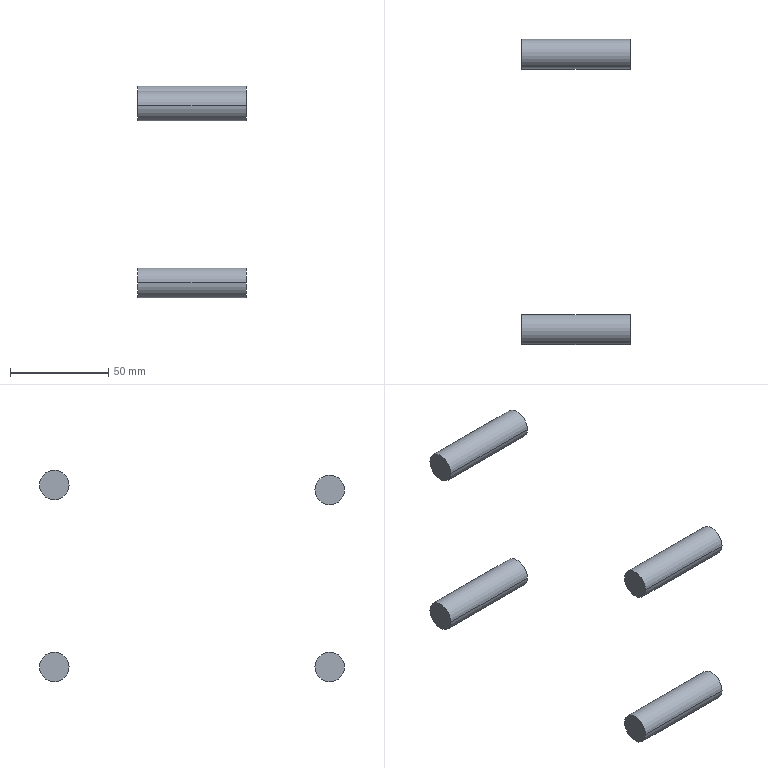Part | STEP file | PN_0012 | 4 solids | 16 faces | box 55 x 155 x 107.5 mm | volume 38877 mm3 | plane 8 | cylinder 8 | commonest cylinder face diameters 15 x8
STEP:
#1=CARTESIAN_POINT('',(0.,0.,0.));
#2=DIRECTION('',(0.,0.,1.));
#3=DIRECTION('',(1.,0.,0.));
#4=AXIS2_PLACEMENT_3D('',#1,#2,#3);
#5=CARTESIAN_POINT('',(124.2,-77.5,47.));
#6=VERTEX_POINT('',#5);
#7=CARTESIAN_POINT('',(124.2,-62.5,47.));
#8=VERTEX_POINT('',#7);
#9=CARTESIAN_POINT('',(124.2,-70.,47.));
#10=DIRECTION('',(-1.,0.,0.));
#11=DIRECTION('',(0.,-1.,0.));
#12=AXIS2_PLACEMENT_3D('',#9,#10,#11);
#13=CIRCLE('',#12,7.5);
#14=CARTESIAN_POINT('',(124.2,0.,0.));
#15=DIRECTION('',(-1.,0.,0.));
#16=DIRECTION('',(0.,-1.,0.));
#17=AXIS2_PLACEMENT_3D('',#14,#15,#16);
#18=PLANE('',#17);
#19=CARTESIAN_POINT('',(70.,47.));
#20=DIRECTION('',(1.,0.));
#21=AXIS2_PLACEMENT_2D('',#19,#20);
#22=CIRCLE('',#21,7.5);
#23=(GEOMETRIC_REPRESENTATION_CONTEXT(2)PARAMETRIC_REPRESENTATION_CONTEXT()REPRESENTATION_CONTEXT('',''));
#24=DEFINITIONAL_REPRESENTATION('',(#22),#23);
#25=PCURVE('',#18,#24);
#26=CARTESIAN_POINT('',(124.2,-70.,47.));
#27=DIRECTION('',(-1.,0.,0.));
#28=DIRECTION('',(0.,-1.,0.));
#29=AXIS2_PLACEMENT_3D('',#26,#27,#28);
#30=CYLINDRICAL_SURFACE('',#29,7.5);
#31=CARTESIAN_POINT('',(0.,0.));
#32=DIRECTION('',(1.,0.));
#33=VECTOR('',#32,1.);
#34=LINE('',#31,#33);
#35=(GEOMETRIC_REPRESENTATION_CONTEXT(2)PARAMETRIC_REPRESENTATION_CONTEXT()REPRESENTATION_CONTEXT('',''));
#36=DEFINITIONAL_REPRESENTATION('',(#34),#35);
#37=PCURVE('',#30,#36);
#38=SURFACE_CURVE('',#13,(#25,#37),.PCURVE_S1.);
#39=EDGE_CURVE('',#6,#8,#38,.T.);
#40=ORIENTED_EDGE('',*,*,#39,.T.);
#41=CARTESIAN_POINT('',(124.2,-70.,47.));
#42=DIRECTION('',(-1.,0.,0.));
#43=DIRECTION('',(0.,1.,0.));
#44=AXIS2_PLACEMENT_3D('',#41,#42,#43);
#45=CIRCLE('',#44,7.5);
#46=CARTESIAN_POINT('',(70.,47.));
#47=DIRECTION('',(-1.,0.));
#48=AXIS2_PLACEMENT_2D('',#46,#47);
#49=CIRCLE('',#48,7.5);
#50=(GEOMETRIC_REPRESENTATION_CONTEXT(2)PARAMETRIC_REPRESENTATION_CONTEXT()REPRESENTATION_CONTEXT('',''));
#51=DEFINITIONAL_REPRESENTATION('',(#49),#50);
#52=PCURVE('',#18,#51);
#53=CARTESIAN_POINT('',(124.2,-70.,47.));
#54=DIRECTION('',(-1.,0.,0.));
#55=DIRECTION('',(0.,-1.,0.));
#56=AXIS2_PLACEMENT_3D('',#53,#54,#55);
#57=CYLINDRICAL_SURFACE('',#56,7.5);
#58=CARTESIAN_POINT('',(3.142,0.));
#59=DIRECTION('',(1.,0.));
#60=VECTOR('',#59,1.);
#61=LINE('',#58,#60);
#62=(GEOMETRIC_REPRESENTATION_CONTEXT(2)PARAMETRIC_REPRESENTATION_CONTEXT()REPRESENTATION_CONTEXT('',''));
#63=DEFINITIONAL_REPRESENTATION('',(#61),#62);
#64=PCURVE('',#57,#63);
#65=SURFACE_CURVE('',#45,(#52,#64),.PCURVE_S1.);
#66=EDGE_CURVE('',#8,#6,#65,.T.);
#67=ORIENTED_EDGE('',*,*,#66,.T.);
#68=EDGE_LOOP('',(#40,#67));
#69=FACE_BOUND('',#68,.F.);
#70=ADVANCED_FACE('',(#69),#18,.F.);
#71=CARTESIAN_POINT('',(69.2,-62.5,47.));
#72=VERTEX_POINT('',#71);
#73=CARTESIAN_POINT('',(124.2,-62.5,47.));
#74=DIRECTION('',(-1.,0.,0.));
#75=VECTOR('',#74,1.);
#76=LINE('',#73,#75);
#77=CARTESIAN_POINT('',(3.142,0.));
#78=DIRECTION('',(0.,1.));
#79=VECTOR('',#78,1.);
#80=LINE('',#77,#79);
#81=(GEOMETRIC_REPRESENTATION_CONTEXT(2)PARAMETRIC_REPRESENTATION_CONTEXT()REPRESENTATION_CONTEXT('',''));
#82=DEFINITIONAL_REPRESENTATION('',(#80),#81);
#83=PCURVE('',#30,#82);
#84=CARTESIAN_POINT('',(3.142,0.));
#85=DIRECTION('',(0.,1.));
#86=VECTOR('',#85,1.);
#87=LINE('',#84,#86);
#88=(GEOMETRIC_REPRESENTATION_CONTEXT(2)PARAMETRIC_REPRESENTATION_CONTEXT()REPRESENTATION_CONTEXT('',''));
#89=DEFINITIONAL_REPRESENTATION('',(#87),#88);
#90=PCURVE('',#57,#89);
#91=SURFACE_CURVE('',#76,(#83,#90),.PCURVE_S1.);
#92=EDGE_CURVE('',#8,#72,#91,.T.);
#93=ORIENTED_EDGE('',*,*,#92,.T.);
#94=CARTESIAN_POINT('',(69.2,-77.5,47.));
#95=VERTEX_POINT('',#94);
#96=CARTESIAN_POINT('',(69.2,-70.,47.));
#97=DIRECTION('',(-1.,0.,0.));
#98=DIRECTION('',(0.,-1.,0.));
#99=AXIS2_PLACEMENT_3D('',#96,#97,#98);
#100=CIRCLE('',#99,7.5);
#101=CARTESIAN_POINT('',(0.,55.));
#102=DIRECTION('',(1.,0.));
#103=VECTOR('',#102,1.);
#104=LINE('',#101,#103);
#105=(GEOMETRIC_REPRESENTATION_CONTEXT(2)PARAMETRIC_REPRESENTATION_CONTEXT()REPRESENTATION_CONTEXT('',''));
#106=DEFINITIONAL_REPRESENTATION('',(#104),#105);
#107=PCURVE('',#30,#106);
#108=CARTESIAN_POINT('',(69.2,0.,0.));
#109=DIRECTION('',(-1.,0.,0.));
#110=DIRECTION('',(0.,-1.,0.));
#111=AXIS2_PLACEMENT_3D('',#108,#109,#110);
#112=PLANE('',#111);
#113=CARTESIAN_POINT('',(70.,47.));
#114=DIRECTION('',(1.,0.));
#115=AXIS2_PLACEMENT_2D('',#113,#114);
#116=CIRCLE('',#115,7.5);
#117=(GEOMETRIC_REPRESENTATION_CONTEXT(2)PARAMETRIC_REPRESENTATION_CONTEXT()REPRESENTATION_CONTEXT('',''));
#118=DEFINITIONAL_REPRESENTATION('',(#116),#117);
#119=PCURVE('',#112,#118);
#120=SURFACE_CURVE('',#100,(#107,#119),.PCURVE_S1.);
#121=EDGE_CURVE('',#95,#72,#120,.T.);
#122=ORIENTED_EDGE('',*,*,#121,.F.);
#123=CARTESIAN_POINT('',(124.2,-77.5,47.));
#124=DIRECTION('',(-1.,0.,0.));
#125=VECTOR('',#124,1.);
#126=LINE('',#123,#125);
#127=CARTESIAN_POINT('',(0.,0.));
#128=DIRECTION('',(0.,1.));
#129=VECTOR('',#128,1.);
#130=LINE('',#127,#129);
#131=(GEOMETRIC_REPRESENTATION_CONTEXT(2)PARAMETRIC_REPRESENTATION_CONTEXT()REPRESENTATION_CONTEXT('',''));
#132=DEFINITIONAL_REPRESENTATION('',(#130),#131);
#133=PCURVE('',#30,#132);
#134=CARTESIAN_POINT('',(6.283,0.));
#135=DIRECTION('',(0.,1.));
#136=VECTOR('',#135,1.);
#137=LINE('',#134,#136);
#138=(GEOMETRIC_REPRESENTATION_CONTEXT(2)PARAMETRIC_REPRESENTATION_CONTEXT()REPRESENTATION_CONTEXT('',''));
#139=DEFINITIONAL_REPRESENTATION('',(#137),#138);
#140=PCURVE('',#57,#139);
#141=SURFACE_CURVE('',#126,(#133,#140),.PCURVE_S1.);
#142=EDGE_CURVE('',#6,#95,#141,.T.);
#143=ORIENTED_EDGE('',*,*,#142,.F.);
#144=ORIENTED_EDGE('',*,*,#39,.T.);
#145=EDGE_LOOP('',(#93,#122,#143,#144));
#146=FACE_BOUND('',#145,.T.);
#147=ADVANCED_FACE('',(#146),#30,.T.);
#148=ORIENTED_EDGE('',*,*,#142,.T.);
#149=CARTESIAN_POINT('',(69.2,-70.,47.));
#150=DIRECTION('',(-1.,0.,0.));
#151=DIRECTION('',(0.,1.,0.));
#152=AXIS2_PLACEMENT_3D('',#149,#150,#151);
#153=CIRCLE('',#152,7.5);
#154=CARTESIAN_POINT('',(3.142,55.));
#155=DIRECTION('',(1.,0.));
#156=VECTOR('',#155,1.);
#157=LINE('',#154,#156);
#158=(GEOMETRIC_REPRESENTATION_CONTEXT(2)PARAMETRIC_REPRESENTATION_CONTEXT()REPRESENTATION_CONTEXT('',''));
#159=DEFINITIONAL_REPRESENTATION('',(#157),#158);
#160=PCURVE('',#57,#159);
#161=CARTESIAN_POINT('',(70.,47.));
#162=DIRECTION('',(-1.,0.));
#163=AXIS2_PLACEMENT_2D('',#161,#162);
#164=CIRCLE('',#163,7.5);
#165=(GEOMETRIC_REPRESENTATION_CONTEXT(2)PARAMETRIC_REPRESENTATION_CONTEXT()REPRESENTATION_CONTEXT('',''));
#166=DEFINITIONAL_REPRESENTATION('',(#164),#165);
#167=PCURVE('',#112,#166);
#168=SURFACE_CURVE('',#153,(#160,#167),.PCURVE_S1.);
#169=EDGE_CURVE('',#72,#95,#168,.T.);
#170=ORIENTED_EDGE('',*,*,#169,.F.);
#171=ORIENTED_EDGE('',*,*,#92,.F.);
#172=ORIENTED_EDGE('',*,*,#66,.T.);
#173=EDGE_LOOP('',(#148,#170,#171,#172));
#174=FACE_BOUND('',#173,.T.);
#175=ADVANCED_FACE('',(#174),#57,.T.);
#176=ORIENTED_EDGE('',*,*,#121,.F.);
#177=ORIENTED_EDGE('',*,*,#169,.F.);
#178=EDGE_LOOP('',(#176,#177));
#179=FACE_BOUND('',#178,.F.);
#180=ADVANCED_FACE('',(#179),#112,.T.);
#181=CLOSED_SHELL('',(#70,#147,#175,#180));
#182=MANIFOLD_SOLID_BREP('',#181);
#183=CARTESIAN_POINT('',(124.2,62.5,49.5));
#184=VERTEX_POINT('',#183);
#185=CARTESIAN_POINT('',(124.2,77.5,49.5));
#186=VERTEX_POINT('',#185);
#187=CARTESIAN_POINT('',(124.2,70.,49.5));
#188=DIRECTION('',(-1.,0.,0.));
#189=DIRECTION('',(0.,-1.,0.));
#190=AXIS2_PLACEMENT_3D('',#187,#188,#189);
#191=CIRCLE('',#190,7.5);
#192=CARTESIAN_POINT('',(124.2,0.,0.));
#193=DIRECTION('',(-1.,0.,0.));
#194=DIRECTION('',(0.,-1.,0.));
#195=AXIS2_PLACEMENT_3D('',#192,#193,#194);
#196=PLANE('',#195);
#197=CARTESIAN_POINT('',(-70.,49.5));
#198=DIRECTION('',(1.,0.));
#199=AXIS2_PLACEMENT_2D('',#197,#198);
#200=CIRCLE('',#199,7.5);
#201=(GEOMETRIC_REPRESENTATION_CONTEXT(2)PARAMETRIC_REPRESENTATION_CONTEXT()REPRESENTATION_CONTEXT('',''));
#202=DEFINITIONAL_REPRESENTATION('',(#200),#201);
#203=PCURVE('',#196,#202);
#204=CARTESIAN_POINT('',(124.2,70.,49.5));
#205=DIRECTION('',(-1.,0.,0.));
#206=DIRECTION('',(0.,-1.,0.));
#207=AXIS2_PLACEMENT_3D('',#204,#205,#206);
#208=CYLINDRICAL_SURFACE('',#207,7.5);
#209=CARTESIAN_POINT('',(0.,0.));
#210=DIRECTION('',(1.,0.));
#211=VECTOR('',#210,1.);
#212=LINE('',#209,#211);
#213=(GEOMETRIC_REPRESENTATION_CONTEXT(2)PARAMETRIC_REPRESENTATION_CONTEXT()REPRESENTATION_CONTEXT('',''));
#214=DEFINITIONAL_REPRESENTATION('',(#212),#213);
#215=PCURVE('',#208,#214);
#216=SURFACE_CURVE('',#191,(#203,#215),.PCURVE_S1.);
#217=EDGE_CURVE('',#184,#186,#216,.T.);
#218=ORIENTED_EDGE('',*,*,#217,.T.);
#219=CARTESIAN_POINT('',(124.2,70.,49.5));
#220=DIRECTION('',(-1.,0.,0.));
#221=DIRECTION('',(0.,1.,0.));
#222=AXIS2_PLACEMENT_3D('',#219,#220,#221);
#223=CIRCLE('',#222,7.5);
#224=CARTESIAN_POINT('',(-70.,49.5));
#225=DIRECTION('',(-1.,0.));
#226=AXIS2_PLACEMENT_2D('',#224,#225);
#227=CIRCLE('',#226,7.5);
#228=(GEOMETRIC_REPRESENTATION_CONTEXT(2)PARAMETRIC_REPRESENTATION_CONTEXT()REPRESENTATION_CONTEXT('',''));
#229=DEFINITIONAL_REPRESENTATION('',(#227),#228);
#230=PCURVE('',#196,#229);
#231=CARTESIAN_POINT('',(124.2,70.,49.5));
#232=DIRECTION('',(-1.,0.,0.));
#233=DIRECTION('',(0.,-1.,0.));
#234=AXIS2_PLACEMENT_3D('',#231,#232,#233);
#235=CYLINDRICAL_SURFACE('',#234,7.5);
#236=CARTESIAN_POINT('',(3.142,0.));
#237=DIRECTION('',(1.,0.));
#238=VECTOR('',#237,1.);
#239=LINE('',#236,#238);
#240=(GEOMETRIC_REPRESENTATION_CONTEXT(2)PARAMETRIC_REPRESENTATION_CONTEXT()REPRESENTATION_CONTEXT('',''));
#241=DEFINITIONAL_REPRESENTATION('',(#239),#240);
#242=PCURVE('',#235,#241);
#243=SURFACE_CURVE('',#223,(#230,#242),.PCURVE_S1.);
#244=EDGE_CURVE('',#186,#184,#243,.T.);
#245=ORIENTED_EDGE('',*,*,#244,.T.);
#246=EDGE_LOOP('',(#218,#245));
#247=FACE_BOUND('',#246,.F.);
#248=ADVANCED_FACE('',(#247),#196,.F.);
#249=CARTESIAN_POINT('',(69.2,77.5,49.5));
#250=VERTEX_POINT('',#249);
#251=CARTESIAN_POINT('',(124.2,77.5,49.5));
#252=DIRECTION('',(-1.,0.,0.));
#253=VECTOR('',#252,1.);
#254=LINE('',#251,#253);
#255=CARTESIAN_POINT('',(3.142,0.));
#256=DIRECTION('',(0.,1.));
#257=VECTOR('',#256,1.);
#258=LINE('',#255,#257);
#259=(GEOMETRIC_REPRESENTATION_CONTEXT(2)PARAMETRIC_REPRESENTATION_CONTEXT()REPRESENTATION_CONTEXT('',''));
#260=DEFINITIONAL_REPRESENTATION('',(#258),#259);
#261=PCURVE('',#208,#260);
#262=CARTESIAN_POINT('',(3.142,0.));
#263=DIRECTION('',(0.,1.));
#264=VECTOR('',#263,1.);
#265=LINE('',#262,#264);
#266=(GEOMETRIC_REPRESENTATION_CONTEXT(2)PARAMETRIC_REPRESENTATION_CONTEXT()REPRESENTATION_CONTEXT('',''));
#267=DEFINITIONAL_REPRESENTATION('',(#265),#266);
#268=PCURVE('',#235,#267);
#269=SURFACE_CURVE('',#254,(#261,#268),.PCURVE_S1.);
#270=EDGE_CURVE('',#186,#250,#269,.T.);
#271=ORIENTED_EDGE('',*,*,#270,.T.);
#272=CARTESIAN_POINT('',(69.2,62.5,49.5));
#273=VERTEX_POINT('',#272);
#274=CARTESIAN_POINT('',(69.2,70.,49.5));
#275=DIRECTION('',(-1.,0.,0.));
#276=DIRECTION('',(0.,-1.,0.));
#277=AXIS2_PLACEMENT_3D('',#274,#275,#276);
#278=CIRCLE('',#277,7.5);
#279=CARTESIAN_POINT('',(0.,55.));
#280=DIRECTION('',(1.,0.));
#281=VECTOR('',#280,1.);
#282=LINE('',#279,#281);
#283=(GEOMETRIC_REPRESENTATION_CONTEXT(2)PARAMETRIC_REPRESENTATION_CONTEXT()REPRESENTATION_CONTEXT('',''));
#284=DEFINITIONAL_REPRESENTATION('',(#282),#283);
#285=PCURVE('',#208,#284);
#286=CARTESIAN_POINT('',(69.2,0.,0.));
#287=DIRECTION('',(-1.,0.,0.));
#288=DIRECTION('',(0.,-1.,0.));
#289=AXIS2_PLACEMENT_3D('',#286,#287,#288);
#290=PLANE('',#289);
#291=CARTESIAN_POINT('',(-70.,49.5));
#292=DIRECTION('',(1.,0.));
#293=AXIS2_PLACEMENT_2D('',#291,#292);
#294=CIRCLE('',#293,7.5);
#295=(GEOMETRIC_REPRESENTATION_CONTEXT(2)PARAMETRIC_REPRESENTATION_CONTEXT()REPRESENTATION_CONTEXT('',''));
#296=DEFINITIONAL_REPRESENTATION('',(#294),#295);
#297=PCURVE('',#290,#296);
#298=SURFACE_CURVE('',#278,(#285,#297),.PCURVE_S1.);
#299=EDGE_CURVE('',#273,#250,#298,.T.);
#300=ORIENTED_EDGE('',*,*,#299,.F.);
#301=CARTESIAN_POINT('',(124.2,62.5,49.5));
#302=DIRECTION('',(-1.,0.,0.));
#303=VECTOR('',#302,1.);
#304=LINE('',#301,#303);
#305=CARTESIAN_POINT('',(0.,0.));
#306=DIRECTION('',(0.,1.));
#307=VECTOR('',#306,1.);
#308=LINE('',#305,#307);
#309=(GEOMETRIC_REPRESENTATION_CONTEXT(2)PARAMETRIC_REPRESENTATION_CONTEXT()REPRESENTATION_CONTEXT('',''));
#310=DEFINITIONAL_REPRESENTATION('',(#308),#309);
#311=PCURVE('',#208,#310);
#312=CARTESIAN_POINT('',(6.283,0.));
#313=DIRECTION('',(0.,1.));
#314=VECTOR('',#313,1.);
#315=LINE('',#312,#314);
#316=(GEOMETRIC_REPRESENTATION_CONTEXT(2)PARAMETRIC_REPRESENTATION_CONTEXT()REPRESENTATION_CONTEXT('',''));
#317=DEFINITIONAL_REPRESENTATION('',(#315),#316);
#318=PCURVE('',#235,#317);
#319=SURFACE_CURVE('',#304,(#311,#318),.PCURVE_S1.);
#320=EDGE_CURVE('',#184,#273,#319,.T.);
#321=ORIENTED_EDGE('',*,*,#320,.F.);
#322=ORIENTED_EDGE('',*,*,#217,.T.);
#323=EDGE_LOOP('',(#271,#300,#321,#322));
#324=FACE_BOUND('',#323,.T.);
#325=ADVANCED_FACE('',(#324),#208,.T.);
#326=ORIENTED_EDGE('',*,*,#320,.T.);
#327=CARTESIAN_POINT('',(69.2,70.,49.5));
#328=DIRECTION('',(-1.,0.,0.));
#329=DIRECTION('',(0.,1.,0.));
#330=AXIS2_PLACEMENT_3D('',#327,#328,#329);
#331=CIRCLE('',#330,7.5);
#332=CARTESIAN_POINT('',(3.142,55.));
#333=DIRECTION('',(1.,0.));
#334=VECTOR('',#333,1.);
#335=LINE('',#332,#334);
#336=(GEOMETRIC_REPRESENTATION_CONTEXT(2)PARAMETRIC_REPRESENTATION_CONTEXT()REPRESENTATION_CONTEXT('',''));
#337=DEFINITIONAL_REPRESENTATION('',(#335),#336);
#338=PCURVE('',#235,#337);
#339=CARTESIAN_POINT('',(-70.,49.5));
#340=DIRECTION('',(-1.,0.));
#341=AXIS2_PLACEMENT_2D('',#339,#340);
#342=CIRCLE('',#341,7.5);
#343=(GEOMETRIC_REPRESENTATION_CONTEXT(2)PARAMETRIC_REPRESENTATION_CONTEXT()REPRESENTATION_CONTEXT('',''));
#344=DEFINITIONAL_REPRESENTATION('',(#342),#343);
#345=PCURVE('',#290,#344);
#346=SURFACE_CURVE('',#331,(#338,#345),.PCURVE_S1.);
#347=EDGE_CURVE('',#250,#273,#346,.T.);
#348=ORIENTED_EDGE('',*,*,#347,.F.);
#349=ORIENTED_EDGE('',*,*,#270,.F.);
#350=ORIENTED_EDGE('',*,*,#244,.T.);
#351=EDGE_LOOP('',(#326,#348,#349,#350));
#352=FACE_BOUND('',#351,.T.);
#353=ADVANCED_FACE('',(#352),#235,.T.);
#354=ORIENTED_EDGE('',*,*,#299,.F.);
#355=ORIENTED_EDGE('',*,*,#347,.F.);
#356=EDGE_LOOP('',(#354,#355));
#357=FACE_BOUND('',#356,.F.);
#358=ADVANCED_FACE('',(#357),#290,.T.);
#359=CLOSED_SHELL('',(#248,#325,#353,#358));
#360=MANIFOLD_SOLID_BREP('',#359);
#361=CARTESIAN_POINT('',(124.2,62.5,-43.));
#362=VERTEX_POINT('',#361);
#363=CARTESIAN_POINT('',(124.2,77.5,-43.));
#364=VERTEX_POINT('',#363);
#365=CARTESIAN_POINT('',(124.2,70.,-43.));
#366=DIRECTION('',(-1.,0.,0.));
#367=DIRECTION('',(0.,-1.,0.));
#368=AXIS2_PLACEMENT_3D('',#365,#366,#367);
#369=CIRCLE('',#368,7.5);
#370=CARTESIAN_POINT('',(124.2,0.,0.));
#371=DIRECTION('',(-1.,0.,0.));
#372=DIRECTION('',(0.,-1.,0.));
#373=AXIS2_PLACEMENT_3D('',#370,#371,#372);
#374=PLANE('',#373);
#375=CARTESIAN_POINT('',(-70.,-43.));
#376=DIRECTION('',(1.,0.));
#377=AXIS2_PLACEMENT_2D('',#375,#376);
#378=CIRCLE('',#377,7.5);
#379=(GEOMETRIC_REPRESENTATION_CONTEXT(2)PARAMETRIC_REPRESENTATION_CONTEXT()REPRESENTATION_CONTEXT('',''));
#380=DEFINITIONAL_REPRESENTATION('',(#378),#379);
#381=PCURVE('',#374,#380);
#382=CARTESIAN_POINT('',(124.2,70.,-43.));
#383=DIRECTION('',(-1.,0.,0.));
#384=DIRECTION('',(0.,-1.,0.));
#385=AXIS2_PLACEMENT_3D('',#382,#383,#384);
#386=CYLINDRICAL_SURFACE('',#385,7.5);
#387=CARTESIAN_POINT('',(0.,0.));
#388=DIRECTION('',(1.,0.));
#389=VECTOR('',#388,1.);
#390=LINE('',#387,#389);
#391=(GEOMETRIC_REPRESENTATION_CONTEXT(2)PARAMETRIC_REPRESENTATION_CONTEXT()REPRESENTATION_CONTEXT('',''));
#392=DEFINITIONAL_REPRESENTATION('',(#390),#391);
#393=PCURVE('',#386,#392);
#394=SURFACE_CURVE('',#369,(#381,#393),.PCURVE_S1.);
#395=EDGE_CURVE('',#362,#364,#394,.T.);
#396=ORIENTED_EDGE('',*,*,#395,.T.);
#397=CARTESIAN_POINT('',(124.2,70.,-43.));
#398=DIRECTION('',(-1.,0.,0.));
#399=DIRECTION('',(0.,1.,0.));
#400=AXIS2_PLACEMENT_3D('',#397,#398,#399);
#401=CIRCLE('',#400,7.5);
#402=CARTESIAN_POINT('',(-70.,-43.));
#403=DIRECTION('',(-1.,0.));
#404=AXIS2_PLACEMENT_2D('',#402,#403);
#405=CIRCLE('',#404,7.5);
#406=(GEOMETRIC_REPRESENTATION_CONTEXT(2)PARAMETRIC_REPRESENTATION_CONTEXT()REPRESENTATION_CONTEXT('',''));
#407=DEFINITIONAL_REPRESENTATION('',(#405),#406);
#408=PCURVE('',#374,#407);
#409=CARTESIAN_POINT('',(124.2,70.,-43.));
#410=DIRECTION('',(-1.,0.,0.));
#411=DIRECTION('',(0.,-1.,0.));
#412=AXIS2_PLACEMENT_3D('',#409,#410,#411);
#413=CYLINDRICAL_SURFACE('',#412,7.5);
#414=CARTESIAN_POINT('',(3.142,0.));
#415=DIRECTION('',(1.,0.));
#416=VECTOR('',#415,1.);
#417=LINE('',#414,#416);
#418=(GEOMETRIC_REPRESENTATION_CONTEXT(2)PARAMETRIC_REPRESENTATION_CONTEXT()REPRESENTATION_CONTEXT('',''));
#419=DEFINITIONAL_REPRESENTATION('',(#417),#418);
#420=PCURVE('',#413,#419);
#421=SURFACE_CURVE('',#401,(#408,#420),.PCURVE_S1.);
#422=EDGE_CURVE('',#364,#362,#421,.T.);
#423=ORIENTED_EDGE('',*,*,#422,.T.);
#424=EDGE_LOOP('',(#396,#423));
#425=FACE_BOUND('',#424,.F.);
#426=ADVANCED_FACE('',(#425),#374,.F.);
#427=CARTESIAN_POINT('',(69.2,77.5,-43.));
#428=VERTEX_POINT('',#427);
#429=CARTESIAN_POINT('',(124.2,77.5,-43.));
#430=DIRECTION('',(-1.,0.,0.));
#431=VECTOR('',#430,1.);
#432=LINE('',#429,#431);
#433=CARTESIAN_POINT('',(3.142,0.));
#434=DIRECTION('',(0.,1.));
#435=VECTOR('',#434,1.);
#436=LINE('',#433,#435);
#437=(GEOMETRIC_REPRESENTATION_CONTEXT(2)PARAMETRIC_REPRESENTATION_CONTEXT()REPRESENTATION_CONTEXT('',''));
#438=DEFINITIONAL_REPRESENTATION('',(#436),#437);
#439=PCURVE('',#386,#438);
#440=CARTESIAN_POINT('',(3.142,0.));
#441=DIRECTION('',(0.,1.));
#442=VECTOR('',#441,1.);
#443=LINE('',#440,#442);
#444=(GEOMETRIC_REPRESENTATION_CONTEXT(2)PARAMETRIC_REPRESENTATION_CONTEXT()REPRESENTATION_CONTEXT('',''));
#445=DEFINITIONAL_REPRESENTATION('',(#443),#444);
#446=PCURVE('',#413,#445);
#447=SURFACE_CURVE('',#432,(#439,#446),.PCURVE_S1.);
#448=EDGE_CURVE('',#364,#428,#447,.T.);
#449=ORIENTED_EDGE('',*,*,#448,.T.);
#450=CARTESIAN_POINT('',(69.2,62.5,-43.));
#451=VERTEX_POINT('',#450);
#452=CARTESIAN_POINT('',(69.2,70.,-43.));
#453=DIRECTION('',(-1.,0.,0.));
#454=DIRECTION('',(0.,-1.,0.));
#455=AXIS2_PLACEMENT_3D('',#452,#453,#454);
#456=CIRCLE('',#455,7.5);
#457=CARTESIAN_POINT('',(0.,55.));
#458=DIRECTION('',(1.,0.));
#459=VECTOR('',#458,1.);
#460=LINE('',#457,#459);
#461=(GEOMETRIC_REPRESENTATION_CONTEXT(2)PARAMETRIC_REPRESENTATION_CONTEXT()REPRESENTATION_CONTEXT('',''));
#462=DEFINITIONAL_REPRESENTATION('',(#460),#461);
#463=PCURVE('',#386,#462);
#464=CARTESIAN_POINT('',(69.2,0.,0.));
#465=DIRECTION('',(-1.,0.,0.));
#466=DIRECTION('',(0.,-1.,0.));
#467=AXIS2_PLACEMENT_3D('',#464,#465,#466);
#468=PLANE('',#467);
#469=CARTESIAN_POINT('',(-70.,-43.));
#470=DIRECTION('',(1.,0.));
#471=AXIS2_PLACEMENT_2D('',#469,#470);
#472=CIRCLE('',#471,7.5);
#473=(GEOMETRIC_REPRESENTATION_CONTEXT(2)PARAMETRIC_REPRESENTATION_CONTEXT()REPRESENTATION_CONTEXT('',''));
#474=DEFINITIONAL_REPRESENTATION('',(#472),#473);
#475=PCURVE('',#468,#474);
#476=SURFACE_CURVE('',#456,(#463,#475),.PCURVE_S1.);
#477=EDGE_CURVE('',#451,#428,#476,.T.);
#478=ORIENTED_EDGE('',*,*,#477,.F.);
#479=CARTESIAN_POINT('',(124.2,62.5,-43.));
#480=DIRECTION('',(-1.,0.,0.));
#481=VECTOR('',#480,1.);
#482=LINE('',#479,#481);
#483=CARTESIAN_POINT('',(0.,0.));
#484=DIRECTION('',(0.,1.));
#485=VECTOR('',#484,1.);
#486=LINE('',#483,#485);
#487=(GEOMETRIC_REPRESENTATION_CONTEXT(2)PARAMETRIC_REPRESENTATION_CONTEXT()REPRESENTATION_CONTEXT('',''));
#488=DEFINITIONAL_REPRESENTATION('',(#486),#487);
#489=PCURVE('',#386,#488);
#490=CARTESIAN_POINT('',(6.283,0.));
#491=DIRECTION('',(0.,1.));
#492=VECTOR('',#491,1.);
#493=LINE('',#490,#492);
#494=(GEOMETRIC_REPRESENTATION_CONTEXT(2)PARAMETRIC_REPRESENTATION_CONTEXT()REPRESENTATION_CONTEXT('',''));
#495=DEFINITIONAL_REPRESENTATION('',(#493),#494);
#496=PCURVE('',#413,#495);
#497=SURFACE_CURVE('',#482,(#489,#496),.PCURVE_S1.);
#498=EDGE_CURVE('',#362,#451,#497,.T.);
#499=ORIENTED_EDGE('',*,*,#498,.F.);
#500=ORIENTED_EDGE('',*,*,#395,.T.);
#501=EDGE_LOOP('',(#449,#478,#499,#500));
#502=FACE_BOUND('',#501,.T.);
#503=ADVANCED_FACE('',(#502),#386,.T.);
#504=ORIENTED_EDGE('',*,*,#498,.T.);
#505=CARTESIAN_POINT('',(69.2,70.,-43.));
#506=DIRECTION('',(-1.,0.,0.));
#507=DIRECTION('',(0.,1.,0.));
#508=AXIS2_PLACEMENT_3D('',#505,#506,#507);
#509=CIRCLE('',#508,7.5);
#510=CARTESIAN_POINT('',(3.142,55.));
#511=DIRECTION('',(1.,0.));
#512=VECTOR('',#511,1.);
#513=LINE('',#510,#512);
#514=(GEOMETRIC_REPRESENTATION_CONTEXT(2)PARAMETRIC_REPRESENTATION_CONTEXT()REPRESENTATION_CONTEXT('',''));
#515=DEFINITIONAL_REPRESENTATION('',(#513),#514);
#516=PCURVE('',#413,#515);
#517=CARTESIAN_POINT('',(-70.,-43.));
#518=DIRECTION('',(-1.,0.));
#519=AXIS2_PLACEMENT_2D('',#517,#518);
#520=CIRCLE('',#519,7.5);
#521=(GEOMETRIC_REPRESENTATION_CONTEXT(2)PARAMETRIC_REPRESENTATION_CONTEXT()REPRESENTATION_CONTEXT('',''));
#522=DEFINITIONAL_REPRESENTATION('',(#520),#521);
#523=PCURVE('',#468,#522);
#524=SURFACE_CURVE('',#509,(#516,#523),.PCURVE_S1.);
#525=EDGE_CURVE('',#428,#451,#524,.T.);
#526=ORIENTED_EDGE('',*,*,#525,.F.);
#527=ORIENTED_EDGE('',*,*,#448,.F.);
#528=ORIENTED_EDGE('',*,*,#422,.T.);
#529=EDGE_LOOP('',(#504,#526,#527,#528));
#530=FACE_BOUND('',#529,.T.);
#531=ADVANCED_FACE('',(#530),#413,.T.);
#532=ORIENTED_EDGE('',*,*,#477,.F.);
#533=ORIENTED_EDGE('',*,*,#525,.F.);
#534=EDGE_LOOP('',(#532,#533));
#535=FACE_BOUND('',#534,.F.);
#536=ADVANCED_FACE('',(#535),#468,.T.);
#537=CLOSED_SHELL('',(#426,#503,#531,#536));
#538=MANIFOLD_SOLID_BREP('',#537);
#539=CARTESIAN_POINT('',(124.2,-77.5,-43.));
#540=VERTEX_POINT('',#539);
#541=CARTESIAN_POINT('',(124.2,-62.5,-43.));
#542=VERTEX_POINT('',#541);
#543=CARTESIAN_POINT('',(124.2,-70.,-43.));
#544=DIRECTION('',(-1.,0.,0.));
#545=DIRECTION('',(0.,-1.,0.));
#546=AXIS2_PLACEMENT_3D('',#543,#544,#545);
#547=CIRCLE('',#546,7.5);
#548=CARTESIAN_POINT('',(124.2,0.,0.));
#549=DIRECTION('',(-1.,0.,0.));
#550=DIRECTION('',(0.,-1.,0.));
#551=AXIS2_PLACEMENT_3D('',#548,#549,#550);
#552=PLANE('',#551);
#553=CARTESIAN_POINT('',(70.,-43.));
#554=DIRECTION('',(1.,0.));
#555=AXIS2_PLACEMENT_2D('',#553,#554);
#556=CIRCLE('',#555,7.5);
#557=(GEOMETRIC_REPRESENTATION_CONTEXT(2)PARAMETRIC_REPRESENTATION_CONTEXT()REPRESENTATION_CONTEXT('',''));
#558=DEFINITIONAL_REPRESENTATION('',(#556),#557);
#559=PCURVE('',#552,#558);
#560=CARTESIAN_POINT('',(124.2,-70.,-43.));
#561=DIRECTION('',(-1.,0.,0.));
#562=DIRECTION('',(0.,-1.,0.));
#563=AXIS2_PLACEMENT_3D('',#560,#561,#562);
#564=CYLINDRICAL_SURFACE('',#563,7.5);
#565=CARTESIAN_POINT('',(0.,0.));
#566=DIRECTION('',(1.,0.));
#567=VECTOR('',#566,1.);
#568=LINE('',#565,#567);
#569=(GEOMETRIC_REPRESENTATION_CONTEXT(2)PARAMETRIC_REPRESENTATION_CONTEXT()REPRESENTATION_CONTEXT('',''));
#570=DEFINITIONAL_REPRESENTATION('',(#568),#569);
#571=PCURVE('',#564,#570);
#572=SURFACE_CURVE('',#547,(#559,#571),.PCURVE_S1.);
#573=EDGE_CURVE('',#540,#542,#572,.T.);
#574=ORIENTED_EDGE('',*,*,#573,.T.);
#575=CARTESIAN_POINT('',(124.2,-70.,-43.));
#576=DIRECTION('',(-1.,0.,0.));
#577=DIRECTION('',(0.,1.,0.));
#578=AXIS2_PLACEMENT_3D('',#575,#576,#577);
#579=CIRCLE('',#578,7.5);
#580=CARTESIAN_POINT('',(70.,-43.));
#581=DIRECTION('',(-1.,0.));
#582=AXIS2_PLACEMENT_2D('',#580,#581);
#583=CIRCLE('',#582,7.5);
#584=(GEOMETRIC_REPRESENTATION_CONTEXT(2)PARAMETRIC_REPRESENTATION_CONTEXT()REPRESENTATION_CONTEXT('',''));
#585=DEFINITIONAL_REPRESENTATION('',(#583),#584);
#586=PCURVE('',#552,#585);
#587=CARTESIAN_POINT('',(124.2,-70.,-43.));
#588=DIRECTION('',(-1.,0.,0.));
#589=DIRECTION('',(0.,-1.,0.));
#590=AXIS2_PLACEMENT_3D('',#587,#588,#589);
#591=CYLINDRICAL_SURFACE('',#590,7.5);
#592=CARTESIAN_POINT('',(3.142,0.));
#593=DIRECTION('',(1.,0.));
#594=VECTOR('',#593,1.);
#595=LINE('',#592,#594);
#596=(GEOMETRIC_REPRESENTATION_CONTEXT(2)PARAMETRIC_REPRESENTATION_CONTEXT()REPRESENTATION_CONTEXT('',''));
#597=DEFINITIONAL_REPRESENTATION('',(#595),#596);
#598=PCURVE('',#591,#597);
#599=SURFACE_CURVE('',#579,(#586,#598),.PCURVE_S1.);
#600=EDGE_CURVE('',#542,#540,#599,.T.);
#601=ORIENTED_EDGE('',*,*,#600,.T.);
#602=EDGE_LOOP('',(#574,#601));
#603=FACE_BOUND('',#602,.F.);
#604=ADVANCED_FACE('',(#603),#552,.F.);
#605=CARTESIAN_POINT('',(69.2,-62.5,-43.));
#606=VERTEX_POINT('',#605);
#607=CARTESIAN_POINT('',(124.2,-62.5,-43.));
#608=DIRECTION('',(-1.,0.,0.));
#609=VECTOR('',#608,1.);
#610=LINE('',#607,#609);
#611=CARTESIAN_POINT('',(3.142,0.));
#612=DIRECTION('',(0.,1.));
#613=VECTOR('',#612,1.);
#614=LINE('',#611,#613);
#615=(GEOMETRIC_REPRESENTATION_CONTEXT(2)PARAMETRIC_REPRESENTATION_CONTEXT()REPRESENTATION_CONTEXT('',''));
#616=DEFINITIONAL_REPRESENTATION('',(#614),#615);
#617=PCURVE('',#564,#616);
#618=CARTESIAN_POINT('',(3.142,0.));
#619=DIRECTION('',(0.,1.));
#620=VECTOR('',#619,1.);
#621=LINE('',#618,#620);
#622=(GEOMETRIC_REPRESENTATION_CONTEXT(2)PARAMETRIC_REPRESENTATION_CONTEXT()REPRESENTATION_CONTEXT('',''));
#623=DEFINITIONAL_REPRESENTATION('',(#621),#622);
#624=PCURVE('',#591,#623);
#625=SURFACE_CURVE('',#610,(#617,#624),.PCURVE_S1.);
#626=EDGE_CURVE('',#542,#606,#625,.T.);
#627=ORIENTED_EDGE('',*,*,#626,.T.);
#628=CARTESIAN_POINT('',(69.2,-77.5,-43.));
#629=VERTEX_POINT('',#628);
#630=CARTESIAN_POINT('',(69.2,-70.,-43.));
#631=DIRECTION('',(-1.,0.,0.));
#632=DIRECTION('',(0.,-1.,0.));
#633=AXIS2_PLACEMENT_3D('',#630,#631,#632);
#634=CIRCLE('',#633,7.5);
#635=CARTESIAN_POINT('',(0.,55.));
#636=DIRECTION('',(1.,0.));
#637=VECTOR('',#636,1.);
#638=LINE('',#635,#637);
#639=(GEOMETRIC_REPRESENTATION_CONTEXT(2)PARAMETRIC_REPRESENTATION_CONTEXT()REPRESENTATION_CONTEXT('',''));
#640=DEFINITIONAL_REPRESENTATION('',(#638),#639);
#641=PCURVE('',#564,#640);
#642=CARTESIAN_POINT('',(69.2,0.,0.));
#643=DIRECTION('',(-1.,0.,0.));
#644=DIRECTION('',(0.,-1.,0.));
#645=AXIS2_PLACEMENT_3D('',#642,#643,#644);
#646=PLANE('',#645);
#647=CARTESIAN_POINT('',(70.,-43.));
#648=DIRECTION('',(1.,0.));
#649=AXIS2_PLACEMENT_2D('',#647,#648);
#650=CIRCLE('',#649,7.5);
#651=(GEOMETRIC_REPRESENTATION_CONTEXT(2)PARAMETRIC_REPRESENTATION_CONTEXT()REPRESENTATION_CONTEXT('',''));
#652=DEFINITIONAL_REPRESENTATION('',(#650),#651);
#653=PCURVE('',#646,#652);
#654=SURFACE_CURVE('',#634,(#641,#653),.PCURVE_S1.);
#655=EDGE_CURVE('',#629,#606,#654,.T.);
#656=ORIENTED_EDGE('',*,*,#655,.F.);
#657=CARTESIAN_POINT('',(124.2,-77.5,-43.));
#658=DIRECTION('',(-1.,0.,0.));
#659=VECTOR('',#658,1.);
#660=LINE('',#657,#659);
#661=CARTESIAN_POINT('',(0.,0.));
#662=DIRECTION('',(0.,1.));
#663=VECTOR('',#662,1.);
#664=LINE('',#661,#663);
#665=(GEOMETRIC_REPRESENTATION_CONTEXT(2)PARAMETRIC_REPRESENTATION_CONTEXT()REPRESENTATION_CONTEXT('',''));
#666=DEFINITIONAL_REPRESENTATION('',(#664),#665);
#667=PCURVE('',#564,#666);
#668=CARTESIAN_POINT('',(6.283,0.));
#669=DIRECTION('',(0.,1.));
#670=VECTOR('',#669,1.);
#671=LINE('',#668,#670);
#672=(GEOMETRIC_REPRESENTATION_CONTEXT(2)PARAMETRIC_REPRESENTATION_CONTEXT()REPRESENTATION_CONTEXT('',''));
#673=DEFINITIONAL_REPRESENTATION('',(#671),#672);
#674=PCURVE('',#591,#673);
#675=SURFACE_CURVE('',#660,(#667,#674),.PCURVE_S1.);
#676=EDGE_CURVE('',#540,#629,#675,.T.);
#677=ORIENTED_EDGE('',*,*,#676,.F.);
#678=ORIENTED_EDGE('',*,*,#573,.T.);
#679=EDGE_LOOP('',(#627,#656,#677,#678));
#680=FACE_BOUND('',#679,.T.);
#681=ADVANCED_FACE('',(#680),#564,.T.);
#682=ORIENTED_EDGE('',*,*,#676,.T.);
#683=CARTESIAN_POINT('',(69.2,-70.,-43.));
#684=DIRECTION('',(-1.,0.,0.));
#685=DIRECTION('',(0.,1.,0.));
#686=AXIS2_PLACEMENT_3D('',#683,#684,#685);
#687=CIRCLE('',#686,7.5);
#688=CARTESIAN_POINT('',(3.142,55.));
#689=DIRECTION('',(1.,0.));
#690=VECTOR('',#689,1.);
#691=LINE('',#688,#690);
#692=(GEOMETRIC_REPRESENTATION_CONTEXT(2)PARAMETRIC_REPRESENTATION_CONTEXT()REPRESENTATION_CONTEXT('',''));
#693=DEFINITIONAL_REPRESENTATION('',(#691),#692);
#694=PCURVE('',#591,#693);
#695=CARTESIAN_POINT('',(70.,-43.));
#696=DIRECTION('',(-1.,0.));
#697=AXIS2_PLACEMENT_2D('',#695,#696);
#698=CIRCLE('',#697,7.5);
#699=(GEOMETRIC_REPRESENTATION_CONTEXT(2)PARAMETRIC_REPRESENTATION_CONTEXT()REPRESENTATION_CONTEXT('',''));
#700=DEFINITIONAL_REPRESENTATION('',(#698),#699);
#701=PCURVE('',#646,#700);
#702=SURFACE_CURVE('',#687,(#694,#701),.PCURVE_S1.);
#703=EDGE_CURVE('',#606,#629,#702,.T.);
#704=ORIENTED_EDGE('',*,*,#703,.F.);
#705=ORIENTED_EDGE('',*,*,#626,.F.);
#706=ORIENTED_EDGE('',*,*,#600,.T.);
#707=EDGE_LOOP('',(#682,#704,#705,#706));
#708=FACE_BOUND('',#707,.T.);
#709=ADVANCED_FACE('',(#708),#591,.T.);
#710=ORIENTED_EDGE('',*,*,#655,.F.);
#711=ORIENTED_EDGE('',*,*,#703,.F.);
#712=EDGE_LOOP('',(#710,#711));
#713=FACE_BOUND('',#712,.F.);
#714=ADVANCED_FACE('',(#713),#646,.T.);
#715=CLOSED_SHELL('',(#604,#681,#709,#714));
#716=MANIFOLD_SOLID_BREP('',#715);
#717=(LENGTH_UNIT()NAMED_UNIT(*)SI_UNIT(.MILLI.,.METRE.));
#718=UNCERTAINTY_MEASURE_WITH_UNIT(LENGTH_MEASURE(0.0000001),#717,'','');
#719=(NAMED_UNIT(*)PLANE_ANGLE_UNIT()SI_UNIT($,.RADIAN.));
#720=(NAMED_UNIT(*)SI_UNIT($,.STERADIAN.)SOLID_ANGLE_UNIT());
#721=(GEOMETRIC_REPRESENTATION_CONTEXT(3)GLOBAL_UNCERTAINTY_ASSIGNED_CONTEXT((#718))GLOBAL_UNIT_ASSIGNED_CONTEXT((#717,#719,#720))REPRESENTATION_CONTEXT('',''));
#722=SHAPE_REPRESENTATION('',(#4,#182,#360,#538,#716),#721);